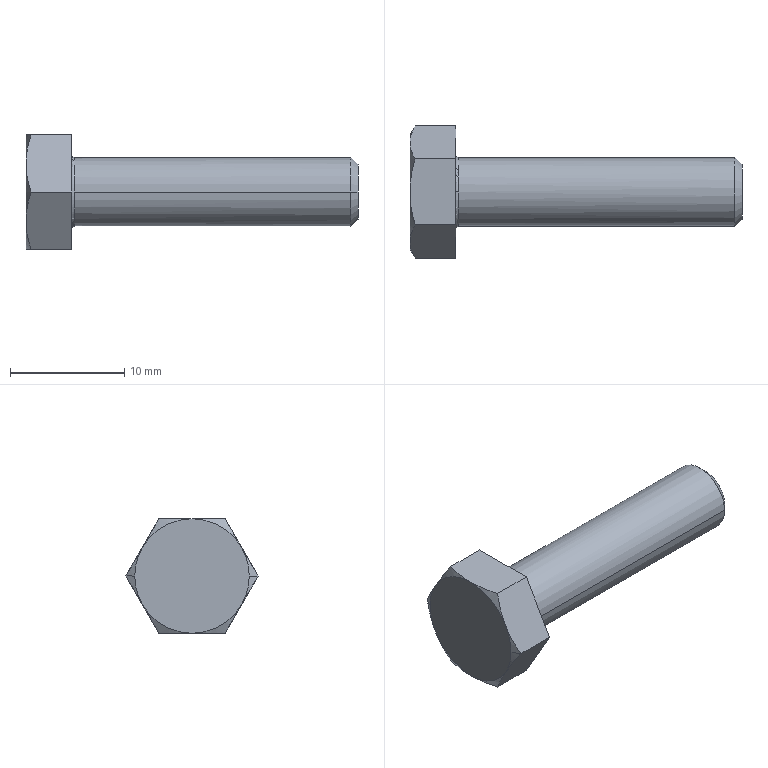Part | STEP file | KS B 1002 - C  M 6 x 25 | 1 solid | 23 faces | box 29 x 11.547 x 10 mm | volume 1049 mm3 | cone 10 | plane 9 | torus 2 | cylinder 2 | commonest cylinder face diameters 6 x2